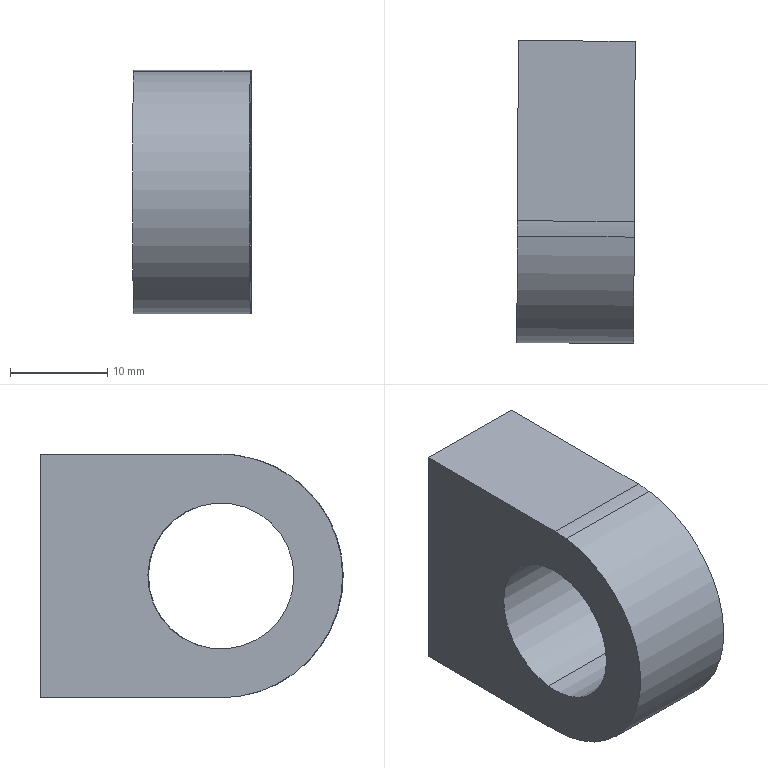Part | STEP file | 2026.6.15-Main Assembly图.sldasm-Part-93 | 1 solid | 14 faces | box 12.158 x 31.061 x 25 mm | volume 6272 mm3 | cylinder 6 | plane 6 | cone 2 | commonest cylinder face diameters 15 x2 17.5 x2 25 x2
STEP:
#1=CARTESIAN_POINT('',(-1541.16,1344.555,3788.748));
#2=VERTEX_POINT('',#1);
#3=CARTESIAN_POINT('',(-1541.149,1346.802,3771.393));
#4=VERTEX_POINT('',#3);
#5=CARTESIAN_POINT('',(-1541.154,1345.678,3780.071));
#6=DIRECTION('',(1.,-0.005111,0.));
#7=DIRECTION('',(-0.0006563,-0.1284,0.9917));
#8=AXIS2_PLACEMENT_3D('',#5,#6,#7);
#9=CIRCLE('',#8,8.75);
#10=EDGE_CURVE('',#2,#4,#9,.T.);
#11=ORIENTED_EDGE('',*,*,#10,.F.);
#12=CARTESIAN_POINT('',(-1540.66,1344.488,3789.244));
#13=VERTEX_POINT('',#12);
#14=CARTESIAN_POINT('',(-1540.66,1344.488,3789.244));
#15=DIRECTION('',(0.7066,-0.09442,0.7013));
#16=VECTOR('',#15,1000.);
#17=LINE('',#14,#16);
#18=EDGE_CURVE('',#2,#13,#17,.T.);
#19=ORIENTED_EDGE('',*,*,#18,.T.);
#20=CARTESIAN_POINT('',(-1540.648,1346.864,3770.897));
#21=VERTEX_POINT('',#20);
#22=CARTESIAN_POINT('',(-1540.654,1345.676,3780.071));
#23=DIRECTION('',(-1.,0.005111,0.));
#24=DIRECTION('',(-0.0006563,-0.1284,0.9917));
#25=AXIS2_PLACEMENT_3D('',#22,#23,#24);
#26=CIRCLE('',#25,9.25);
#27=EDGE_CURVE('',#21,#13,#26,.T.);
#28=ORIENTED_EDGE('',*,*,#27,.F.);
#29=CARTESIAN_POINT('',(-1540.648,1346.864,3770.897));
#30=DIRECTION('',(0.7076,0.08719,-0.7013));
#31=VECTOR('',#30,1000.);
#32=LINE('',#29,#31);
#33=EDGE_CURVE('',#4,#21,#32,.T.);
#34=ORIENTED_EDGE('',*,*,#33,.F.);
#35=EDGE_LOOP('',(#11,#19,#28,#34));
#36=FACE_OUTER_BOUND('',#35,.T.);
#37=CARTESIAN_POINT('',(-1540.654,1345.676,3780.071));
#38=DIRECTION('',(1.,-0.005111,0.));
#39=DIRECTION('',(0.0006563,0.1284,-0.9917));
#40=AXIS2_PLACEMENT_3D('',#37,#38,#39);
#41=CONICAL_SURFACE('',#40,9.25,0.7854);
#42=ADVANCED_FACE('',(#36),#41,.F.);
#43=CARTESIAN_POINT('',(-1542.16,1344.56,3788.748));
#44=VERTEX_POINT('',#43);
#45=CARTESIAN_POINT('',(-1542.149,1346.807,3771.393));
#46=VERTEX_POINT('',#45);
#47=CARTESIAN_POINT('',(-1542.154,1345.683,3780.071));
#48=DIRECTION('',(1.,-0.005111,0.));
#49=DIRECTION('',(-0.0006563,-0.1284,0.9917));
#50=AXIS2_PLACEMENT_3D('',#47,#48,#49);
#51=CIRCLE('',#50,8.75);
#52=EDGE_CURVE('',#44,#46,#51,.T.);
#53=ORIENTED_EDGE('',*,*,#52,.F.);
#54=CARTESIAN_POINT('',(-1542.16,1344.56,3788.748));
#55=DIRECTION('',(1.,-0.005111,0.));
#56=VECTOR('',#55,1000.);
#57=LINE('',#54,#56);
#58=EDGE_CURVE('',#44,#2,#57,.T.);
#59=ORIENTED_EDGE('',*,*,#58,.T.);
#60=ORIENTED_EDGE('',*,*,#10,.T.);
#61=CARTESIAN_POINT('',(-1542.149,1346.807,3771.393));
#62=DIRECTION('',(1.,-0.005111,0.));
#63=VECTOR('',#62,1000.);
#64=LINE('',#61,#63);
#65=EDGE_CURVE('',#46,#4,#64,.T.);
#66=ORIENTED_EDGE('',*,*,#65,.F.);
#67=EDGE_LOOP('',(#53,#59,#60,#66));
#68=FACE_OUTER_BOUND('',#67,.T.);
#69=CARTESIAN_POINT('',(-1542.154,1345.683,3780.071));
#70=DIRECTION('',(1.,-0.005111,0.));
#71=DIRECTION('',(0.0006563,0.1284,-0.9917));
#72=AXIS2_PLACEMENT_3D('',#69,#70,#71);
#73=CYLINDRICAL_SURFACE('',#72,8.75);
#74=ADVANCED_FACE('',(#68),#73,.F.);
#75=CARTESIAN_POINT('',(-1542.149,1346.646,3772.633));
#76=VERTEX_POINT('',#75);
#77=CARTESIAN_POINT('',(-1542.159,1344.72,3787.509));
#78=VERTEX_POINT('',#77);
#79=CARTESIAN_POINT('',(-1542.154,1345.683,3780.071));
#80=DIRECTION('',(-1.,0.005111,0.));
#81=DIRECTION('',(-0.0006563,-0.1284,0.9917));
#82=AXIS2_PLACEMENT_3D('',#79,#80,#81);
#83=CIRCLE('',#82,7.5);
#84=EDGE_CURVE('',#76,#78,#83,.T.);
#85=ORIENTED_EDGE('',*,*,#84,.F.);
#86=CARTESIAN_POINT('',(-1552.649,1346.7,3772.633));
#87=VERTEX_POINT('',#86);
#88=CARTESIAN_POINT('',(-1540.649,1346.639,3772.633));
#89=DIRECTION('',(-1.,0.005111,0.));
#90=VECTOR('',#89,1000.);
#91=LINE('',#88,#90);
#92=EDGE_CURVE('',#76,#87,#91,.T.);
#93=ORIENTED_EDGE('',*,*,#92,.T.);
#94=CARTESIAN_POINT('',(-1552.659,1344.774,3787.509));
#95=VERTEX_POINT('',#94);
#96=CARTESIAN_POINT('',(-1552.654,1345.737,3780.071));
#97=DIRECTION('',(1.,-0.005111,0.));
#98=DIRECTION('',(0.005111,1.,0.));
#99=AXIS2_PLACEMENT_3D('',#96,#97,#98);
#100=CIRCLE('',#99,7.5);
#101=EDGE_CURVE('',#95,#87,#100,.T.);
#102=ORIENTED_EDGE('',*,*,#101,.F.);
#103=CARTESIAN_POINT('',(-1540.659,1344.713,3787.509));
#104=DIRECTION('',(-1.,0.005111,0.));
#105=VECTOR('',#104,1000.);
#106=LINE('',#103,#105);
#107=EDGE_CURVE('',#78,#95,#106,.T.);
#108=ORIENTED_EDGE('',*,*,#107,.F.);
#109=EDGE_LOOP('',(#85,#93,#102,#108));
#110=FACE_OUTER_BOUND('',#109,.T.);
#111=CARTESIAN_POINT('',(-1540.654,1345.676,3780.071));
#112=DIRECTION('',(-1.,0.005111,0.));
#113=DIRECTION('',(-0.0006563,-0.1284,0.9917));
#114=AXIS2_PLACEMENT_3D('',#111,#112,#113);
#115=CYLINDRICAL_SURFACE('',#114,7.5);
#116=ADVANCED_FACE('',(#110),#115,.F.);
#117=CARTESIAN_POINT('',(-1540.654,1345.676,3767.571));
#118=VERTEX_POINT('',#117);
#119=CARTESIAN_POINT('',(-1540.663,1344.071,3792.467));
#120=VERTEX_POINT('',#119);
#121=CARTESIAN_POINT('',(-1540.654,1345.676,3780.071));
#122=DIRECTION('',(-1.,0.005111,0.));
#123=DIRECTION('',(0.005111,1.,0.));
#124=AXIS2_PLACEMENT_3D('',#121,#122,#123);
#125=CIRCLE('',#124,12.5);
#126=EDGE_CURVE('',#118,#120,#125,.T.);
#127=ORIENTED_EDGE('',*,*,#126,.T.);
#128=CARTESIAN_POINT('',(-1552.662,1344.132,3792.467));
#129=VERTEX_POINT('',#128);
#130=CARTESIAN_POINT('',(-1540.663,1344.071,3792.467));
#131=DIRECTION('',(-1.,0.005111,0.));
#132=VECTOR('',#131,1000.);
#133=LINE('',#130,#132);
#134=EDGE_CURVE('',#120,#129,#133,.T.);
#135=ORIENTED_EDGE('',*,*,#134,.T.);
#136=CARTESIAN_POINT('',(-1552.654,1345.737,3767.571));
#137=VERTEX_POINT('',#136);
#138=CARTESIAN_POINT('',(-1552.654,1345.737,3780.071));
#139=DIRECTION('',(-1.,0.005111,0.));
#140=DIRECTION('',(0.005111,1.,0.));
#141=AXIS2_PLACEMENT_3D('',#138,#139,#140);
#142=CIRCLE('',#141,12.5);
#143=EDGE_CURVE('',#137,#129,#142,.T.);
#144=ORIENTED_EDGE('',*,*,#143,.F.);
#145=CARTESIAN_POINT('',(-1540.654,1345.676,3767.571));
#146=DIRECTION('',(-1.,0.005111,0.));
#147=VECTOR('',#146,1000.);
#148=LINE('',#145,#147);
#149=EDGE_CURVE('',#118,#137,#148,.T.);
#150=ORIENTED_EDGE('',*,*,#149,.F.);
#151=EDGE_LOOP('',(#127,#135,#144,#150));
#152=FACE_OUTER_BOUND('',#151,.T.);
#153=CARTESIAN_POINT('',(-1540.654,1345.676,3780.071));
#154=DIRECTION('',(-1.,0.005111,0.));
#155=DIRECTION('',(-0.0006563,-0.1284,0.9917));
#156=AXIS2_PLACEMENT_3D('',#153,#154,#155);
#157=CYLINDRICAL_SURFACE('',#156,12.5);
#158=ADVANCED_FACE('',(#152),#157,.T.);
#159=CARTESIAN_POINT('',(-1552.56,1364.237,3767.571));
#160=VERTEX_POINT('',#159);
#161=CARTESIAN_POINT('',(-1552.56,1364.237,3767.571));
#162=DIRECTION('',(-0.005111,-1.,0.));
#163=VECTOR('',#162,1000.);
#164=LINE('',#161,#163);
#165=EDGE_CURVE('',#160,#137,#164,.T.);
#166=ORIENTED_EDGE('',*,*,#165,.F.);
#167=CARTESIAN_POINT('',(-1540.56,1364.175,3767.571));
#168=VERTEX_POINT('',#167);
#169=CARTESIAN_POINT('',(-1540.56,1364.175,3767.571));
#170=DIRECTION('',(-1.,0.005111,0.));
#171=VECTOR('',#170,1000.);
#172=LINE('',#169,#171);
#173=EDGE_CURVE('',#168,#160,#172,.T.);
#174=ORIENTED_EDGE('',*,*,#173,.F.);
#175=CARTESIAN_POINT('',(-1540.56,1364.175,3767.571));
#176=DIRECTION('',(-0.005111,-1.,0.));
#177=VECTOR('',#176,1000.);
#178=LINE('',#175,#177);
#179=EDGE_CURVE('',#168,#118,#178,.T.);
#180=ORIENTED_EDGE('',*,*,#179,.T.);
#181=ORIENTED_EDGE('',*,*,#149,.T.);
#182=EDGE_LOOP('',(#166,#174,#180,#181));
#183=FACE_OUTER_BOUND('',#182,.T.);
#184=CARTESIAN_POINT('',(-1540.56,1364.175,3767.571));
#185=DIRECTION('',(0.,0.,-1.));
#186=DIRECTION('',(0.0007664,1.,0.));
#187=AXIS2_PLACEMENT_3D('',#184,#185,#186);
#188=PLANE('',#187);
#189=ADVANCED_FACE('',(#183),#188,.T.);
#190=ORIENTED_EDGE('',*,*,#134,.F.);
#191=CARTESIAN_POINT('',(-1540.654,1345.676,3792.571));
#192=VERTEX_POINT('',#191);
#193=CARTESIAN_POINT('',(-1540.654,1345.676,3780.071));
#194=DIRECTION('',(-1.,0.005111,0.));
#195=DIRECTION('',(0.005111,1.,0.));
#196=AXIS2_PLACEMENT_3D('',#193,#194,#195);
#197=CIRCLE('',#196,12.5);
#198=EDGE_CURVE('',#120,#192,#197,.T.);
#199=ORIENTED_EDGE('',*,*,#198,.T.);
#200=CARTESIAN_POINT('',(-1552.654,1345.737,3792.571));
#201=VERTEX_POINT('',#200);
#202=CARTESIAN_POINT('',(-1540.654,1345.676,3792.571));
#203=DIRECTION('',(-1.,0.005111,0.));
#204=VECTOR('',#203,1000.);
#205=LINE('',#202,#204);
#206=EDGE_CURVE('',#192,#201,#205,.T.);
#207=ORIENTED_EDGE('',*,*,#206,.T.);
#208=CARTESIAN_POINT('',(-1552.654,1345.737,3780.071));
#209=DIRECTION('',(-1.,0.005111,0.));
#210=DIRECTION('',(0.005111,1.,0.));
#211=AXIS2_PLACEMENT_3D('',#208,#209,#210);
#212=CIRCLE('',#211,12.5);
#213=EDGE_CURVE('',#129,#201,#212,.T.);
#214=ORIENTED_EDGE('',*,*,#213,.F.);
#215=EDGE_LOOP('',(#190,#199,#207,#214));
#216=FACE_OUTER_BOUND('',#215,.T.);
#217=CARTESIAN_POINT('',(-1540.654,1345.676,3780.071));
#218=DIRECTION('',(-1.,0.005111,0.));
#219=DIRECTION('',(-0.0006563,-0.1284,0.9917));
#220=AXIS2_PLACEMENT_3D('',#217,#218,#219);
#221=CYLINDRICAL_SURFACE('',#220,12.5);
#222=ADVANCED_FACE('',(#216),#221,.T.);
#223=CARTESIAN_POINT('',(-1552.56,1364.237,3792.571));
#224=VERTEX_POINT('',#223);
#225=CARTESIAN_POINT('',(-1552.654,1345.737,3792.571));
#226=DIRECTION('',(0.005111,1.,0.));
#227=VECTOR('',#226,1000.);
#228=LINE('',#225,#227);
#229=EDGE_CURVE('',#201,#224,#228,.T.);
#230=ORIENTED_EDGE('',*,*,#229,.F.);
#231=ORIENTED_EDGE('',*,*,#206,.F.);
#232=CARTESIAN_POINT('',(-1540.56,1364.175,3792.571));
#233=VERTEX_POINT('',#232);
#234=CARTESIAN_POINT('',(-1540.654,1345.676,3792.571));
#235=DIRECTION('',(0.005111,1.,0.));
#236=VECTOR('',#235,1000.);
#237=LINE('',#234,#236);
#238=EDGE_CURVE('',#192,#233,#237,.T.);
#239=ORIENTED_EDGE('',*,*,#238,.T.);
#240=CARTESIAN_POINT('',(-1540.56,1364.175,3792.571));
#241=DIRECTION('',(-1.,0.005111,0.));
#242=VECTOR('',#241,1000.);
#243=LINE('',#240,#242);
#244=EDGE_CURVE('',#233,#224,#243,.T.);
#245=ORIENTED_EDGE('',*,*,#244,.T.);
#246=EDGE_LOOP('',(#230,#231,#239,#245));
#247=FACE_OUTER_BOUND('',#246,.T.);
#248=CARTESIAN_POINT('',(-1540.654,1345.676,3792.571));
#249=DIRECTION('',(0.,0.,1.));
#250=DIRECTION('',(-0.0007664,-1.,0.));
#251=AXIS2_PLACEMENT_3D('',#248,#249,#250);
#252=PLANE('',#251);
#253=ADVANCED_FACE('',(#247),#252,.T.);
#254=CARTESIAN_POINT('',(-1552.56,1364.237,3792.571));
#255=DIRECTION('',(0.,0.,-1.));
#256=VECTOR('',#255,1000.);
#257=LINE('',#254,#256);
#258=EDGE_CURVE('',#224,#160,#257,.T.);
#259=ORIENTED_EDGE('',*,*,#258,.F.);
#260=ORIENTED_EDGE('',*,*,#244,.F.);
#261=CARTESIAN_POINT('',(-1540.56,1364.175,3792.571));
#262=DIRECTION('',(0.,0.,-1.));
#263=VECTOR('',#262,1000.);
#264=LINE('',#261,#263);
#265=EDGE_CURVE('',#233,#168,#264,.T.);
#266=ORIENTED_EDGE('',*,*,#265,.T.);
#267=ORIENTED_EDGE('',*,*,#173,.T.);
#268=EDGE_LOOP('',(#259,#260,#266,#267));
#269=FACE_OUTER_BOUND('',#268,.T.);
#270=CARTESIAN_POINT('',(-1540.56,1364.175,3792.571));
#271=DIRECTION('',(0.005111,1.,0.));
#272=DIRECTION('',(0.03353,-0.0001714,0.9994));
#273=AXIS2_PLACEMENT_3D('',#270,#271,#272);
#274=PLANE('',#273);
#275=ADVANCED_FACE('',(#269),#274,.T.);
#276=ORIENTED_EDGE('',*,*,#92,.F.);
#277=CARTESIAN_POINT('',(-1542.154,1345.683,3780.071));
#278=DIRECTION('',(-1.,0.005111,0.));
#279=DIRECTION('',(-0.0006563,-0.1284,0.9917));
#280=AXIS2_PLACEMENT_3D('',#277,#278,#279);
#281=CIRCLE('',#280,7.5);
#282=EDGE_CURVE('',#78,#76,#281,.T.);
#283=ORIENTED_EDGE('',*,*,#282,.F.);
#284=ORIENTED_EDGE('',*,*,#107,.T.);
#285=CARTESIAN_POINT('',(-1552.654,1345.737,3780.071));
#286=DIRECTION('',(1.,-0.005111,0.));
#287=DIRECTION('',(0.005111,1.,0.));
#288=AXIS2_PLACEMENT_3D('',#285,#286,#287);
#289=CIRCLE('',#288,7.5);
#290=EDGE_CURVE('',#87,#95,#289,.T.);
#291=ORIENTED_EDGE('',*,*,#290,.F.);
#292=EDGE_LOOP('',(#276,#283,#284,#291));
#293=FACE_OUTER_BOUND('',#292,.T.);
#294=CARTESIAN_POINT('',(-1540.654,1345.676,3780.071));
#295=DIRECTION('',(-1.,0.005111,0.));
#296=DIRECTION('',(-0.0006563,-0.1284,0.9917));
#297=AXIS2_PLACEMENT_3D('',#294,#295,#296);
#298=CYLINDRICAL_SURFACE('',#297,7.5);
#299=ADVANCED_FACE('',(#293),#298,.F.);
#300=ORIENTED_EDGE('',*,*,#27,.T.);
#301=CARTESIAN_POINT('',(-1540.654,1345.676,3780.071));
#302=DIRECTION('',(-1.,0.005111,0.));
#303=DIRECTION('',(-0.0006563,-0.1284,0.9917));
#304=AXIS2_PLACEMENT_3D('',#301,#302,#303);
#305=CIRCLE('',#304,9.25);
#306=EDGE_CURVE('',#13,#21,#305,.T.);
#307=ORIENTED_EDGE('',*,*,#306,.T.);
#308=EDGE_LOOP('',(#300,#307));
#309=FACE_BOUND('',#308,.T.);
#310=ORIENTED_EDGE('',*,*,#179,.F.);
#311=ORIENTED_EDGE('',*,*,#265,.F.);
#312=ORIENTED_EDGE('',*,*,#238,.F.);
#313=ORIENTED_EDGE('',*,*,#198,.F.);
#314=ORIENTED_EDGE('',*,*,#126,.F.);
#315=EDGE_LOOP('',(#310,#311,#312,#313,#314));
#316=FACE_OUTER_BOUND('',#315,.T.);
#317=CARTESIAN_POINT('',(-1540.654,1345.676,3780.071));
#318=DIRECTION('',(-1.,0.005111,0.));
#319=DIRECTION('',(-0.0006563,-0.1284,0.9917));
#320=AXIS2_PLACEMENT_3D('',#317,#318,#319);
#321=PLANE('',#320);
#322=ADVANCED_FACE('',(#309,#316),#321,.F.);
#323=ORIENTED_EDGE('',*,*,#165,.T.);
#324=ORIENTED_EDGE('',*,*,#143,.T.);
#325=ORIENTED_EDGE('',*,*,#213,.T.);
#326=ORIENTED_EDGE('',*,*,#229,.T.);
#327=ORIENTED_EDGE('',*,*,#258,.T.);
#328=EDGE_LOOP('',(#323,#324,#325,#326,#327));
#329=FACE_OUTER_BOUND('',#328,.T.);
#330=ORIENTED_EDGE('',*,*,#101,.T.);
#331=ORIENTED_EDGE('',*,*,#290,.T.);
#332=EDGE_LOOP('',(#330,#331));
#333=FACE_BOUND('',#332,.T.);
#334=CARTESIAN_POINT('',(-1552.654,1345.737,3780.071));
#335=DIRECTION('',(-1.,0.005111,0.));
#336=DIRECTION('',(-0.0006563,-0.1284,0.9917));
#337=AXIS2_PLACEMENT_3D('',#334,#335,#336);
#338=PLANE('',#337);
#339=ADVANCED_FACE('',(#329,#333),#338,.T.);
#340=ORIENTED_EDGE('',*,*,#58,.F.);
#341=CARTESIAN_POINT('',(-1542.154,1345.683,3780.071));
#342=DIRECTION('',(1.,-0.005111,0.));
#343=DIRECTION('',(-0.0006563,-0.1284,0.9917));
#344=AXIS2_PLACEMENT_3D('',#341,#342,#343);
#345=CIRCLE('',#344,8.75);
#346=EDGE_CURVE('',#46,#44,#345,.T.);
#347=ORIENTED_EDGE('',*,*,#346,.F.);
#348=ORIENTED_EDGE('',*,*,#65,.T.);
#349=CARTESIAN_POINT('',(-1541.154,1345.678,3780.071));
#350=DIRECTION('',(1.,-0.005111,0.));
#351=DIRECTION('',(-0.0006563,-0.1284,0.9917));
#352=AXIS2_PLACEMENT_3D('',#349,#350,#351);
#353=CIRCLE('',#352,8.75);
#354=EDGE_CURVE('',#4,#2,#353,.T.);
#355=ORIENTED_EDGE('',*,*,#354,.T.);
#356=EDGE_LOOP('',(#340,#347,#348,#355));
#357=FACE_OUTER_BOUND('',#356,.T.);
#358=CARTESIAN_POINT('',(-1542.154,1345.683,3780.071));
#359=DIRECTION('',(1.,-0.005111,0.));
#360=DIRECTION('',(0.0006563,0.1284,-0.9917));
#361=AXIS2_PLACEMENT_3D('',#358,#359,#360);
#362=CYLINDRICAL_SURFACE('',#361,8.75);
#363=ADVANCED_FACE('',(#357),#362,.F.);
#364=ORIENTED_EDGE('',*,*,#282,.T.);
#365=ORIENTED_EDGE('',*,*,#84,.T.);
#366=EDGE_LOOP('',(#364,#365));
#367=FACE_BOUND('',#366,.T.);
#368=ORIENTED_EDGE('',*,*,#346,.T.);
#369=ORIENTED_EDGE('',*,*,#52,.T.);
#370=EDGE_LOOP('',(#368,#369));
#371=FACE_OUTER_BOUND('',#370,.T.);
#372=CARTESIAN_POINT('',(-1542.154,1345.683,3780.071));
#373=DIRECTION('',(-1.,0.005111,0.));
#374=DIRECTION('',(-0.0006563,-0.1284,0.9917));
#375=AXIS2_PLACEMENT_3D('',#372,#373,#374);
#376=PLANE('',#375);
#377=ADVANCED_FACE('',(#367,#371),#376,.F.);
#378=ORIENTED_EDGE('',*,*,#18,.F.);
#379=ORIENTED_EDGE('',*,*,#354,.F.);
#380=ORIENTED_EDGE('',*,*,#33,.T.);
#381=ORIENTED_EDGE('',*,*,#306,.F.);
#382=EDGE_LOOP('',(#378,#379,#380,#381));
#383=FACE_OUTER_BOUND('',#382,.T.);
#384=CARTESIAN_POINT('',(-1540.654,1345.676,3780.071));
#385=DIRECTION('',(1.,-0.005111,0.));
#386=DIRECTION('',(0.0006563,0.1284,-0.9917));
#387=AXIS2_PLACEMENT_3D('',#384,#385,#386);
#388=CONICAL_SURFACE('',#387,9.25,0.7854);
#389=ADVANCED_FACE('',(#383),#388,.F.);
#390=CLOSED_SHELL('',(#42,#74,#116,#158,#189,#222,#253,#275,#299,#322,#339,#363,#377,#389));
#391=MANIFOLD_SOLID_BREP('',#390);
#392=CARTESIAN_POINT('',(0.,0.,0.));
#393=DIRECTION('',(0.,0.,1.));
#394=DIRECTION('',(1.,0.,0.));
#395=AXIS2_PLACEMENT_3D('',#392,#393,#394);
#396=(LENGTH_UNIT()NAMED_UNIT(*)SI_UNIT(.MILLI.,.METRE.));
#397=UNCERTAINTY_MEASURE_WITH_UNIT(LENGTH_MEASURE(0.00001),#396,'','');
#398=(NAMED_UNIT(*)PLANE_ANGLE_UNIT()SI_UNIT($,.RADIAN.));
#399=(NAMED_UNIT(*)SI_UNIT($,.STERADIAN.)SOLID_ANGLE_UNIT());
#400=(GEOMETRIC_REPRESENTATION_CONTEXT(3)GLOBAL_UNCERTAINTY_ASSIGNED_CONTEXT((#397))GLOBAL_UNIT_ASSIGNED_CONTEXT((#396,#398,#399))REPRESENTATION_CONTEXT('',''));
#401=ADVANCED_BREP_SHAPE_REPRESENTATION('',(#391,#395),#400);